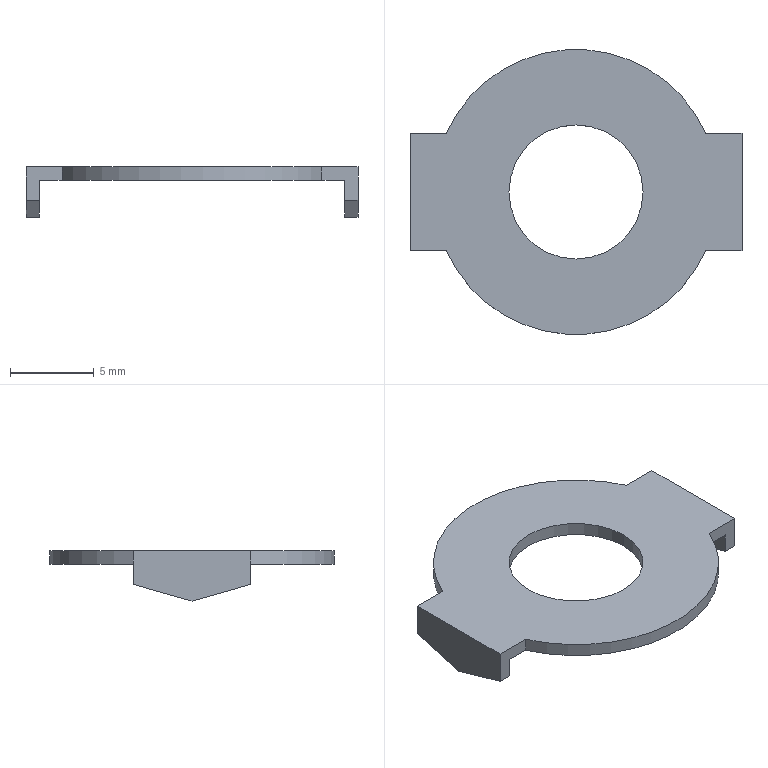Part | SolidWorks | features BaseBody 1 | 1 solid | 18 faces | box 19.8 x 17 x 3 mm | volume 178.855 mm3 | plane 14 | cylinder 4 | commonest cylinder face diameters 8 x2 17 x2
STEP:
#1=CARTESIAN_POINT('',(-4.,0.,-0.8));
#2=VERTEX_POINT('',#1);
#3=CARTESIAN_POINT('',(4.,0.,-0.8));
#4=VERTEX_POINT('',#3);
#5=CARTESIAN_POINT('',(0.,0.,-0.8));
#6=DIRECTION('',(0.,0.,1.));
#7=DIRECTION('',(1.,0.,0.));
#8=AXIS2_PLACEMENT_3D('',#5,#6,#7);
#9=CIRCLE('',#8,4.);
#10=EDGE_CURVE('',#2,#4,#9,.T.);
#11=ORIENTED_EDGE('',*,*,#10,.F.);
#12=CARTESIAN_POINT('',(-4.,0.,0.));
#13=VERTEX_POINT('',#12);
#14=CARTESIAN_POINT('',(-4.,0.,-3.));
#15=DIRECTION('',(0.,0.,1.));
#16=VECTOR('',#15,1000.);
#17=LINE('',#14,#16);
#18=EDGE_CURVE('',#2,#13,#17,.T.);
#19=ORIENTED_EDGE('',*,*,#18,.T.);
#20=CARTESIAN_POINT('',(4.,0.,0.));
#21=VERTEX_POINT('',#20);
#22=CARTESIAN_POINT('',(0.,0.,0.));
#23=DIRECTION('',(0.,0.,1.));
#24=DIRECTION('',(1.,0.,0.));
#25=AXIS2_PLACEMENT_3D('',#22,#23,#24);
#26=CIRCLE('',#25,4.);
#27=EDGE_CURVE('',#13,#21,#26,.T.);
#28=ORIENTED_EDGE('',*,*,#27,.T.);
#29=CARTESIAN_POINT('',(4.,0.,-3.));
#30=DIRECTION('',(0.,0.,1.));
#31=VECTOR('',#30,1000.);
#32=LINE('',#29,#31);
#33=EDGE_CURVE('',#4,#21,#32,.T.);
#34=ORIENTED_EDGE('',*,*,#33,.F.);
#35=EDGE_LOOP('',(#11,#19,#28,#34));
#36=FACE_OUTER_BOUND('',#35,.T.);
#37=CARTESIAN_POINT('',(0.,0.,-3.));
#38=DIRECTION('',(0.,0.,1.));
#39=DIRECTION('',(1.,0.,0.));
#40=AXIS2_PLACEMENT_3D('',#37,#38,#39);
#41=CYLINDRICAL_SURFACE('',#40,4.);
#42=ADVANCED_FACE('',(#36),#41,.F.);
#43=CARTESIAN_POINT('',(0.,0.,-0.8));
#44=DIRECTION('',(0.,0.,1.));
#45=DIRECTION('',(1.,0.,0.));
#46=AXIS2_PLACEMENT_3D('',#43,#44,#45);
#47=CIRCLE('',#46,4.);
#48=EDGE_CURVE('',#4,#2,#47,.T.);
#49=ORIENTED_EDGE('',*,*,#48,.T.);
#50=ORIENTED_EDGE('',*,*,#10,.T.);
#51=EDGE_LOOP('',(#49,#50));
#52=FACE_BOUND('',#51,.T.);
#53=CARTESIAN_POINT('',(-9.1,3.5,-0.8));
#54=VERTEX_POINT('',#53);
#55=CARTESIAN_POINT('',(-9.1,-3.5,-0.8));
#56=VERTEX_POINT('',#55);
#57=CARTESIAN_POINT('',(-9.1,0.,-0.8));
#58=DIRECTION('',(0.,-1.,0.));
#59=VECTOR('',#58,1000.);
#60=LINE('',#57,#59);
#61=EDGE_CURVE('',#54,#56,#60,.T.);
#62=ORIENTED_EDGE('',*,*,#61,.F.);
#63=CARTESIAN_POINT('',(-7.746,3.5,-0.8));
#64=VERTEX_POINT('',#63);
#65=CARTESIAN_POINT('',(-9.9,3.5,-0.8));
#66=DIRECTION('',(-1.,0.,0.));
#67=VECTOR('',#66,1000.);
#68=LINE('',#65,#67);
#69=EDGE_CURVE('',#64,#54,#68,.T.);
#70=ORIENTED_EDGE('',*,*,#69,.F.);
#71=CARTESIAN_POINT('',(7.746,3.5,-0.8));
#72=VERTEX_POINT('',#71);
#73=CARTESIAN_POINT('',(0.,0.,-0.8));
#74=DIRECTION('',(0.,0.,1.));
#75=DIRECTION('',(1.,0.,0.));
#76=AXIS2_PLACEMENT_3D('',#73,#74,#75);
#77=CIRCLE('',#76,8.5);
#78=EDGE_CURVE('',#72,#64,#77,.T.);
#79=ORIENTED_EDGE('',*,*,#78,.F.);
#80=CARTESIAN_POINT('',(9.1,3.5,-0.8));
#81=VERTEX_POINT('',#80);
#82=CARTESIAN_POINT('',(7.746,3.5,-0.8));
#83=DIRECTION('',(-1.,0.,0.));
#84=VECTOR('',#83,1000.);
#85=LINE('',#82,#84);
#86=EDGE_CURVE('',#81,#72,#85,.T.);
#87=ORIENTED_EDGE('',*,*,#86,.F.);
#88=CARTESIAN_POINT('',(9.1,-3.5,-0.8));
#89=VERTEX_POINT('',#88);
#90=CARTESIAN_POINT('',(9.1,0.,-0.8));
#91=DIRECTION('',(0.,1.,0.));
#92=VECTOR('',#91,1000.);
#93=LINE('',#90,#92);
#94=EDGE_CURVE('',#89,#81,#93,.T.);
#95=ORIENTED_EDGE('',*,*,#94,.F.);
#96=CARTESIAN_POINT('',(7.746,-3.5,-0.8));
#97=VERTEX_POINT('',#96);
#98=CARTESIAN_POINT('',(7.746,-3.5,-0.8));
#99=DIRECTION('',(1.,0.,0.));
#100=VECTOR('',#99,1000.);
#101=LINE('',#98,#100);
#102=EDGE_CURVE('',#97,#89,#101,.T.);
#103=ORIENTED_EDGE('',*,*,#102,.F.);
#104=CARTESIAN_POINT('',(-7.746,-3.5,-0.8));
#105=VERTEX_POINT('',#104);
#106=CARTESIAN_POINT('',(0.,0.,-0.8));
#107=DIRECTION('',(0.,0.,1.));
#108=DIRECTION('',(1.,0.,0.));
#109=AXIS2_PLACEMENT_3D('',#106,#107,#108);
#110=CIRCLE('',#109,8.5);
#111=EDGE_CURVE('',#105,#97,#110,.T.);
#112=ORIENTED_EDGE('',*,*,#111,.F.);
#113=CARTESIAN_POINT('',(-9.9,-3.5,-0.8));
#114=DIRECTION('',(1.,0.,0.));
#115=VECTOR('',#114,1000.);
#116=LINE('',#113,#115);
#117=EDGE_CURVE('',#56,#105,#116,.T.);
#118=ORIENTED_EDGE('',*,*,#117,.F.);
#119=EDGE_LOOP('',(#62,#70,#79,#87,#95,#103,#112,#118));
#120=FACE_OUTER_BOUND('',#119,.T.);
#121=CARTESIAN_POINT('',(0.,0.,-0.8));
#122=DIRECTION('',(0.,0.,1.));
#123=DIRECTION('',(1.,0.,0.));
#124=AXIS2_PLACEMENT_3D('',#121,#122,#123);
#125=PLANE('',#124);
#126=ADVANCED_FACE('',(#52,#120),#125,.F.);
#127=CARTESIAN_POINT('',(-7.746,-3.5,0.));
#128=VERTEX_POINT('',#127);
#129=CARTESIAN_POINT('',(7.746,-3.5,0.));
#130=VERTEX_POINT('',#129);
#131=CARTESIAN_POINT('',(0.,0.,0.));
#132=DIRECTION('',(0.,0.,1.));
#133=DIRECTION('',(1.,0.,0.));
#134=AXIS2_PLACEMENT_3D('',#131,#132,#133);
#135=CIRCLE('',#134,8.5);
#136=EDGE_CURVE('',#128,#130,#135,.T.);
#137=ORIENTED_EDGE('',*,*,#136,.F.);
#138=CARTESIAN_POINT('',(-7.746,-3.5,-0.8));
#139=DIRECTION('',(0.,0.,1.));
#140=VECTOR('',#139,1000.);
#141=LINE('',#138,#140);
#142=EDGE_CURVE('',#105,#128,#141,.T.);
#143=ORIENTED_EDGE('',*,*,#142,.F.);
#144=ORIENTED_EDGE('',*,*,#111,.T.);
#145=CARTESIAN_POINT('',(7.746,-3.5,-0.8));
#146=DIRECTION('',(0.,0.,1.));
#147=VECTOR('',#146,1000.);
#148=LINE('',#145,#147);
#149=EDGE_CURVE('',#97,#130,#148,.T.);
#150=ORIENTED_EDGE('',*,*,#149,.T.);
#151=EDGE_LOOP('',(#137,#143,#144,#150));
#152=FACE_OUTER_BOUND('',#151,.T.);
#153=CARTESIAN_POINT('',(0.,0.,-0.8));
#154=DIRECTION('',(0.,0.,1.));
#155=DIRECTION('',(1.,0.,0.));
#156=AXIS2_PLACEMENT_3D('',#153,#154,#155);
#157=CYLINDRICAL_SURFACE('',#156,8.5);
#158=ADVANCED_FACE('',(#152),#157,.T.);
#159=CARTESIAN_POINT('',(-9.9,-3.5,-2.));
#160=VERTEX_POINT('',#159);
#161=CARTESIAN_POINT('',(-9.9,-3.5,0.));
#162=VERTEX_POINT('',#161);
#163=CARTESIAN_POINT('',(-9.9,-3.5,-0.8));
#164=DIRECTION('',(0.,0.,1.));
#165=VECTOR('',#164,1000.);
#166=LINE('',#163,#165);
#167=EDGE_CURVE('',#160,#162,#166,.T.);
#168=ORIENTED_EDGE('',*,*,#167,.F.);
#169=CARTESIAN_POINT('',(-9.1,-3.5,-2.));
#170=VERTEX_POINT('',#169);
#171=CARTESIAN_POINT('',(-9.1,-3.5,-2.));
#172=DIRECTION('',(-1.,0.,0.));
#173=VECTOR('',#172,1000.);
#174=LINE('',#171,#173);
#175=EDGE_CURVE('',#170,#160,#174,.T.);
#176=ORIENTED_EDGE('',*,*,#175,.F.);
#177=CARTESIAN_POINT('',(-9.1,-3.5,0.));
#178=DIRECTION('',(0.,0.,-1.));
#179=VECTOR('',#178,1000.);
#180=LINE('',#177,#179);
#181=EDGE_CURVE('',#56,#170,#180,.T.);
#182=ORIENTED_EDGE('',*,*,#181,.F.);
#183=ORIENTED_EDGE('',*,*,#117,.T.);
#184=ORIENTED_EDGE('',*,*,#142,.T.);
#185=CARTESIAN_POINT('',(-9.9,-3.5,0.));
#186=DIRECTION('',(1.,0.,0.));
#187=VECTOR('',#186,1000.);
#188=LINE('',#185,#187);
#189=EDGE_CURVE('',#162,#128,#188,.T.);
#190=ORIENTED_EDGE('',*,*,#189,.F.);
#191=EDGE_LOOP('',(#168,#176,#182,#183,#184,#190));
#192=FACE_OUTER_BOUND('',#191,.T.);
#193=CARTESIAN_POINT('',(-9.9,-3.5,-0.8));
#194=DIRECTION('',(0.,-1.,0.));
#195=DIRECTION('',(1.,0.,0.));
#196=AXIS2_PLACEMENT_3D('',#193,#194,#195);
#197=PLANE('',#196);
#198=ADVANCED_FACE('',(#192),#197,.T.);
#199=CARTESIAN_POINT('',(-9.9,3.5,0.));
#200=VERTEX_POINT('',#199);
#201=CARTESIAN_POINT('',(-9.9,3.5,0.));
#202=DIRECTION('',(0.,-1.,0.));
#203=VECTOR('',#202,1000.);
#204=LINE('',#201,#203);
#205=EDGE_CURVE('',#200,#162,#204,.T.);
#206=ORIENTED_EDGE('',*,*,#205,.F.);
#207=CARTESIAN_POINT('',(-9.9,3.5,-2.));
#208=VERTEX_POINT('',#207);
#209=CARTESIAN_POINT('',(-9.9,3.5,-0.8));
#210=DIRECTION('',(0.,0.,1.));
#211=VECTOR('',#210,1000.);
#212=LINE('',#209,#211);
#213=EDGE_CURVE('',#208,#200,#212,.T.);
#214=ORIENTED_EDGE('',*,*,#213,.F.);
#215=CARTESIAN_POINT('',(-9.9,0.,-3.));
#216=VERTEX_POINT('',#215);
#217=CARTESIAN_POINT('',(-9.9,3.5,-2.));
#218=DIRECTION('',(0.,0.9615,0.2747));
#219=VECTOR('',#218,1000.);
#220=LINE('',#217,#219);
#221=EDGE_CURVE('',#216,#208,#220,.T.);
#222=ORIENTED_EDGE('',*,*,#221,.F.);
#223=CARTESIAN_POINT('',(-9.9,-3.5,-2.));
#224=DIRECTION('',(0.,0.9615,-0.2747));
#225=VECTOR('',#224,1000.);
#226=LINE('',#223,#225);
#227=EDGE_CURVE('',#160,#216,#226,.T.);
#228=ORIENTED_EDGE('',*,*,#227,.F.);
#229=ORIENTED_EDGE('',*,*,#167,.T.);
#230=EDGE_LOOP('',(#206,#214,#222,#228,#229));
#231=FACE_OUTER_BOUND('',#230,.T.);
#232=CARTESIAN_POINT('',(-9.9,3.5,-0.8));
#233=DIRECTION('',(-1.,0.,0.));
#234=DIRECTION('',(0.,0.,1.));
#235=AXIS2_PLACEMENT_3D('',#232,#233,#234);
#236=PLANE('',#235);
#237=ADVANCED_FACE('',(#231),#236,.T.);
#238=ORIENTED_EDGE('',*,*,#213,.T.);
#239=CARTESIAN_POINT('',(-7.746,3.5,0.));
#240=VERTEX_POINT('',#239);
#241=CARTESIAN_POINT('',(-9.9,3.5,0.));
#242=DIRECTION('',(-1.,0.,0.));
#243=VECTOR('',#242,1000.);
#244=LINE('',#241,#243);
#245=EDGE_CURVE('',#240,#200,#244,.T.);
#246=ORIENTED_EDGE('',*,*,#245,.F.);
#247=CARTESIAN_POINT('',(-7.746,3.5,-0.8));
#248=DIRECTION('',(0.,0.,1.));
#249=VECTOR('',#248,1000.);
#250=LINE('',#247,#249);
#251=EDGE_CURVE('',#64,#240,#250,.T.);
#252=ORIENTED_EDGE('',*,*,#251,.F.);
#253=ORIENTED_EDGE('',*,*,#69,.T.);
#254=CARTESIAN_POINT('',(-9.1,3.5,-2.));
#255=VERTEX_POINT('',#254);
#256=CARTESIAN_POINT('',(-9.1,3.5,0.));
#257=DIRECTION('',(0.,0.,1.));
#258=VECTOR('',#257,1000.);
#259=LINE('',#256,#258);
#260=EDGE_CURVE('',#255,#54,#259,.T.);
#261=ORIENTED_EDGE('',*,*,#260,.F.);
#262=CARTESIAN_POINT('',(-9.1,3.5,-2.));
#263=DIRECTION('',(-1.,0.,0.));
#264=VECTOR('',#263,1000.);
#265=LINE('',#262,#264);
#266=EDGE_CURVE('',#255,#208,#265,.T.);
#267=ORIENTED_EDGE('',*,*,#266,.T.);
#268=EDGE_LOOP('',(#238,#246,#252,#253,#261,#267));
#269=FACE_OUTER_BOUND('',#268,.T.);
#270=CARTESIAN_POINT('',(-9.9,3.5,-0.8));
#271=DIRECTION('',(0.,1.,0.));
#272=DIRECTION('',(-1.,0.,0.));
#273=AXIS2_PLACEMENT_3D('',#270,#271,#272);
#274=PLANE('',#273);
#275=ADVANCED_FACE('',(#269),#274,.T.);
#276=CARTESIAN_POINT('',(7.746,3.5,0.));
#277=VERTEX_POINT('',#276);
#278=CARTESIAN_POINT('',(0.,0.,0.));
#279=DIRECTION('',(0.,0.,1.));
#280=DIRECTION('',(1.,0.,0.));
#281=AXIS2_PLACEMENT_3D('',#278,#279,#280);
#282=CIRCLE('',#281,8.5);
#283=EDGE_CURVE('',#277,#240,#282,.T.);
#284=ORIENTED_EDGE('',*,*,#283,.F.);
#285=CARTESIAN_POINT('',(7.746,3.5,-0.8));
#286=DIRECTION('',(0.,0.,1.));
#287=VECTOR('',#286,1000.);
#288=LINE('',#285,#287);
#289=EDGE_CURVE('',#72,#277,#288,.T.);
#290=ORIENTED_EDGE('',*,*,#289,.F.);
#291=ORIENTED_EDGE('',*,*,#78,.T.);
#292=ORIENTED_EDGE('',*,*,#251,.T.);
#293=EDGE_LOOP('',(#284,#290,#291,#292));
#294=FACE_OUTER_BOUND('',#293,.T.);
#295=CARTESIAN_POINT('',(0.,0.,-0.8));
#296=DIRECTION('',(0.,0.,1.));
#297=DIRECTION('',(1.,0.,0.));
#298=AXIS2_PLACEMENT_3D('',#295,#296,#297);
#299=CYLINDRICAL_SURFACE('',#298,8.5);
#300=ADVANCED_FACE('',(#294),#299,.T.);
#301=CARTESIAN_POINT('',(9.1,3.5,-2.));
#302=VERTEX_POINT('',#301);
#303=CARTESIAN_POINT('',(9.1,3.5,0.));
#304=DIRECTION('',(0.,0.,1.));
#305=VECTOR('',#304,1000.);
#306=LINE('',#303,#305);
#307=EDGE_CURVE('',#302,#81,#306,.T.);
#308=ORIENTED_EDGE('',*,*,#307,.T.);
#309=ORIENTED_EDGE('',*,*,#86,.T.);
#310=ORIENTED_EDGE('',*,*,#289,.T.);
#311=CARTESIAN_POINT('',(9.9,3.5,0.));
#312=VERTEX_POINT('',#311);
#313=CARTESIAN_POINT('',(7.746,3.5,0.));
#314=DIRECTION('',(-1.,0.,0.));
#315=VECTOR('',#314,1000.);
#316=LINE('',#313,#315);
#317=EDGE_CURVE('',#312,#277,#316,.T.);
#318=ORIENTED_EDGE('',*,*,#317,.F.);
#319=CARTESIAN_POINT('',(9.9,3.5,-2.));
#320=VERTEX_POINT('',#319);
#321=CARTESIAN_POINT('',(9.9,3.5,-0.8));
#322=DIRECTION('',(0.,0.,1.));
#323=VECTOR('',#322,1000.);
#324=LINE('',#321,#323);
#325=EDGE_CURVE('',#320,#312,#324,.T.);
#326=ORIENTED_EDGE('',*,*,#325,.F.);
#327=CARTESIAN_POINT('',(9.1,3.5,-2.));
#328=DIRECTION('',(1.,0.,0.));
#329=VECTOR('',#328,1000.);
#330=LINE('',#327,#329);
#331=EDGE_CURVE('',#302,#320,#330,.T.);
#332=ORIENTED_EDGE('',*,*,#331,.F.);
#333=EDGE_LOOP('',(#308,#309,#310,#318,#326,#332));
#334=FACE_OUTER_BOUND('',#333,.T.);
#335=CARTESIAN_POINT('',(7.746,3.5,-0.8));
#336=DIRECTION('',(0.,1.,0.));
#337=DIRECTION('',(-1.,0.,0.));
#338=AXIS2_PLACEMENT_3D('',#335,#336,#337);
#339=PLANE('',#338);
#340=ADVANCED_FACE('',(#334),#339,.T.);
#341=CARTESIAN_POINT('',(9.9,-3.5,0.));
#342=VERTEX_POINT('',#341);
#343=CARTESIAN_POINT('',(9.9,3.5,0.));
#344=DIRECTION('',(0.,1.,0.));
#345=VECTOR('',#344,1000.);
#346=LINE('',#343,#345);
#347=EDGE_CURVE('',#342,#312,#346,.T.);
#348=ORIENTED_EDGE('',*,*,#347,.F.);
#349=CARTESIAN_POINT('',(9.9,-3.5,-2.));
#350=VERTEX_POINT('',#349);
#351=CARTESIAN_POINT('',(9.9,-3.5,-0.8));
#352=DIRECTION('',(0.,0.,1.));
#353=VECTOR('',#352,1000.);
#354=LINE('',#351,#353);
#355=EDGE_CURVE('',#350,#342,#354,.T.);
#356=ORIENTED_EDGE('',*,*,#355,.F.);
#357=CARTESIAN_POINT('',(9.9,0.,-3.));
#358=VERTEX_POINT('',#357);
#359=CARTESIAN_POINT('',(9.9,-3.5,-2.));
#360=DIRECTION('',(0.,0.9615,-0.2747));
#361=VECTOR('',#360,1000.);
#362=LINE('',#359,#361);
#363=EDGE_CURVE('',#350,#358,#362,.T.);
#364=ORIENTED_EDGE('',*,*,#363,.T.);
#365=CARTESIAN_POINT('',(9.9,3.5,-2.));
#366=DIRECTION('',(0.,0.9615,0.2747));
#367=VECTOR('',#366,1000.);
#368=LINE('',#365,#367);
#369=EDGE_CURVE('',#358,#320,#368,.T.);
#370=ORIENTED_EDGE('',*,*,#369,.T.);
#371=ORIENTED_EDGE('',*,*,#325,.T.);
#372=EDGE_LOOP('',(#348,#356,#364,#370,#371));
#373=FACE_OUTER_BOUND('',#372,.T.);
#374=CARTESIAN_POINT('',(9.9,3.5,-0.8));
#375=DIRECTION('',(1.,0.,0.));
#376=DIRECTION('',(0.,0.,-1.));
#377=AXIS2_PLACEMENT_3D('',#374,#375,#376);
#378=PLANE('',#377);
#379=ADVANCED_FACE('',(#373),#378,.T.);
#380=ORIENTED_EDGE('',*,*,#355,.T.);
#381=CARTESIAN_POINT('',(7.746,-3.5,0.));
#382=DIRECTION('',(1.,0.,0.));
#383=VECTOR('',#382,1000.);
#384=LINE('',#381,#383);
#385=EDGE_CURVE('',#130,#342,#384,.T.);
#386=ORIENTED_EDGE('',*,*,#385,.F.);
#387=ORIENTED_EDGE('',*,*,#149,.F.);
#388=ORIENTED_EDGE('',*,*,#102,.T.);
#389=CARTESIAN_POINT('',(9.1,-3.5,-2.));
#390=VERTEX_POINT('',#389);
#391=CARTESIAN_POINT('',(9.1,-3.5,0.));
#392=DIRECTION('',(0.,0.,-1.));
#393=VECTOR('',#392,1000.);
#394=LINE('',#391,#393);
#395=EDGE_CURVE('',#89,#390,#394,.T.);
#396=ORIENTED_EDGE('',*,*,#395,.T.);
#397=CARTESIAN_POINT('',(9.1,-3.5,-2.));
#398=DIRECTION('',(1.,0.,0.));
#399=VECTOR('',#398,1000.);
#400=LINE('',#397,#399);
#401=EDGE_CURVE('',#390,#350,#400,.T.);
#402=ORIENTED_EDGE('',*,*,#401,.T.);
#403=EDGE_LOOP('',(#380,#386,#387,#388,#396,#402));
#404=FACE_OUTER_BOUND('',#403,.T.);
#405=CARTESIAN_POINT('',(7.746,-3.5,-0.8));
#406=DIRECTION('',(0.,-1.,0.));
#407=DIRECTION('',(1.,0.,0.));
#408=AXIS2_PLACEMENT_3D('',#405,#406,#407);
#409=PLANE('',#408);
#410=ADVANCED_FACE('',(#404),#409,.T.);
#411=CARTESIAN_POINT('',(0.,0.,0.));
#412=DIRECTION('',(0.,0.,1.));
#413=DIRECTION('',(1.,0.,0.));
#414=AXIS2_PLACEMENT_3D('',#411,#412,#413);
#415=CIRCLE('',#414,4.);
#416=EDGE_CURVE('',#21,#13,#415,.T.);
#417=ORIENTED_EDGE('',*,*,#416,.F.);
#418=ORIENTED_EDGE('',*,*,#27,.F.);
#419=EDGE_LOOP('',(#417,#418));
#420=FACE_BOUND('',#419,.T.);
#421=ORIENTED_EDGE('',*,*,#189,.T.);
#422=ORIENTED_EDGE('',*,*,#136,.T.);
#423=ORIENTED_EDGE('',*,*,#385,.T.);
#424=ORIENTED_EDGE('',*,*,#347,.T.);
#425=ORIENTED_EDGE('',*,*,#317,.T.);
#426=ORIENTED_EDGE('',*,*,#283,.T.);
#427=ORIENTED_EDGE('',*,*,#245,.T.);
#428=ORIENTED_EDGE('',*,*,#205,.T.);
#429=EDGE_LOOP('',(#421,#422,#423,#424,#425,#426,#427,#428));
#430=FACE_OUTER_BOUND('',#429,.T.);
#431=CARTESIAN_POINT('',(0.,0.,0.));
#432=DIRECTION('',(0.,0.,1.));
#433=DIRECTION('',(1.,0.,0.));
#434=AXIS2_PLACEMENT_3D('',#431,#432,#433);
#435=PLANE('',#434);
#436=ADVANCED_FACE('',(#420,#430),#435,.T.);
#437=ORIENTED_EDGE('',*,*,#395,.F.);
#438=ORIENTED_EDGE('',*,*,#94,.T.);
#439=ORIENTED_EDGE('',*,*,#307,.F.);
#440=CARTESIAN_POINT('',(9.1,0.,-3.));
#441=VERTEX_POINT('',#440);
#442=CARTESIAN_POINT('',(9.1,3.5,-2.));
#443=DIRECTION('',(0.,0.9615,0.2747));
#444=VECTOR('',#443,1000.);
#445=LINE('',#442,#444);
#446=EDGE_CURVE('',#441,#302,#445,.T.);
#447=ORIENTED_EDGE('',*,*,#446,.F.);
#448=CARTESIAN_POINT('',(9.1,-3.5,-2.));
#449=DIRECTION('',(0.,0.9615,-0.2747));
#450=VECTOR('',#449,1000.);
#451=LINE('',#448,#450);
#452=EDGE_CURVE('',#390,#441,#451,.T.);
#453=ORIENTED_EDGE('',*,*,#452,.F.);
#454=EDGE_LOOP('',(#437,#438,#439,#447,#453));
#455=FACE_OUTER_BOUND('',#454,.T.);
#456=CARTESIAN_POINT('',(9.1,-3.5,0.));
#457=DIRECTION('',(1.,0.,0.));
#458=DIRECTION('',(0.,0.,-1.));
#459=AXIS2_PLACEMENT_3D('',#456,#457,#458);
#460=PLANE('',#459);
#461=ADVANCED_FACE('',(#455),#460,.F.);
#462=ORIENTED_EDGE('',*,*,#369,.F.);
#463=CARTESIAN_POINT('',(9.1,0.,-3.));
#464=DIRECTION('',(1.,0.,0.));
#465=VECTOR('',#464,1000.);
#466=LINE('',#463,#465);
#467=EDGE_CURVE('',#441,#358,#466,.T.);
#468=ORIENTED_EDGE('',*,*,#467,.F.);
#469=ORIENTED_EDGE('',*,*,#446,.T.);
#470=ORIENTED_EDGE('',*,*,#331,.T.);
#471=EDGE_LOOP('',(#462,#468,#469,#470));
#472=FACE_OUTER_BOUND('',#471,.T.);
#473=CARTESIAN_POINT('',(9.1,3.5,-2.));
#474=DIRECTION('',(0.,0.2747,-0.9615));
#475=DIRECTION('',(0.,0.9615,0.2747));
#476=AXIS2_PLACEMENT_3D('',#473,#474,#475);
#477=PLANE('',#476);
#478=ADVANCED_FACE('',(#472),#477,.T.);
#479=ORIENTED_EDGE('',*,*,#363,.F.);
#480=ORIENTED_EDGE('',*,*,#401,.F.);
#481=ORIENTED_EDGE('',*,*,#452,.T.);
#482=ORIENTED_EDGE('',*,*,#467,.T.);
#483=EDGE_LOOP('',(#479,#480,#481,#482));
#484=FACE_OUTER_BOUND('',#483,.T.);
#485=CARTESIAN_POINT('',(9.1,-3.5,-2.));
#486=DIRECTION('',(0.,-0.2747,-0.9615));
#487=DIRECTION('',(0.,0.9615,-0.2747));
#488=AXIS2_PLACEMENT_3D('',#485,#486,#487);
#489=PLANE('',#488);
#490=ADVANCED_FACE('',(#484),#489,.T.);
#491=ORIENTED_EDGE('',*,*,#260,.T.);
#492=ORIENTED_EDGE('',*,*,#61,.T.);
#493=ORIENTED_EDGE('',*,*,#181,.T.);
#494=CARTESIAN_POINT('',(-9.1,0.,-3.));
#495=VERTEX_POINT('',#494);
#496=CARTESIAN_POINT('',(-9.1,-3.5,-2.));
#497=DIRECTION('',(0.,0.9615,-0.2747));
#498=VECTOR('',#497,1000.);
#499=LINE('',#496,#498);
#500=EDGE_CURVE('',#170,#495,#499,.T.);
#501=ORIENTED_EDGE('',*,*,#500,.T.);
#502=CARTESIAN_POINT('',(-9.1,3.5,-2.));
#503=DIRECTION('',(0.,0.9615,0.2747));
#504=VECTOR('',#503,1000.);
#505=LINE('',#502,#504);
#506=EDGE_CURVE('',#495,#255,#505,.T.);
#507=ORIENTED_EDGE('',*,*,#506,.T.);
#508=EDGE_LOOP('',(#491,#492,#493,#501,#507));
#509=FACE_OUTER_BOUND('',#508,.T.);
#510=CARTESIAN_POINT('',(-9.1,-3.5,0.));
#511=DIRECTION('',(-1.,0.,0.));
#512=DIRECTION('',(0.,0.,-1.));
#513=AXIS2_PLACEMENT_3D('',#510,#511,#512);
#514=PLANE('',#513);
#515=ADVANCED_FACE('',(#509),#514,.F.);
#516=ORIENTED_EDGE('',*,*,#227,.T.);
#517=CARTESIAN_POINT('',(-9.1,0.,-3.));
#518=DIRECTION('',(-1.,0.,0.));
#519=VECTOR('',#518,1000.);
#520=LINE('',#517,#519);
#521=EDGE_CURVE('',#495,#216,#520,.T.);
#522=ORIENTED_EDGE('',*,*,#521,.F.);
#523=ORIENTED_EDGE('',*,*,#500,.F.);
#524=ORIENTED_EDGE('',*,*,#175,.T.);
#525=EDGE_LOOP('',(#516,#522,#523,#524));
#526=FACE_OUTER_BOUND('',#525,.T.);
#527=CARTESIAN_POINT('',(-9.1,-3.5,-2.));
#528=DIRECTION('',(0.,0.2747,0.9615));
#529=DIRECTION('',(0.,-0.9615,0.2747));
#530=AXIS2_PLACEMENT_3D('',#527,#528,#529);
#531=PLANE('',#530);
#532=ADVANCED_FACE('',(#526),#531,.F.);
#533=ORIENTED_EDGE('',*,*,#221,.T.);
#534=ORIENTED_EDGE('',*,*,#266,.F.);
#535=ORIENTED_EDGE('',*,*,#506,.F.);
#536=ORIENTED_EDGE('',*,*,#521,.T.);
#537=EDGE_LOOP('',(#533,#534,#535,#536));
#538=FACE_OUTER_BOUND('',#537,.T.);
#539=CARTESIAN_POINT('',(-9.1,3.5,-2.));
#540=DIRECTION('',(0.,-0.2747,0.9615));
#541=DIRECTION('',(0.,-0.9615,-0.2747));
#542=AXIS2_PLACEMENT_3D('',#539,#540,#541);
#543=PLANE('',#542);
#544=ADVANCED_FACE('',(#538),#543,.F.);
#545=ORIENTED_EDGE('',*,*,#18,.F.);
#546=ORIENTED_EDGE('',*,*,#48,.F.);
#547=ORIENTED_EDGE('',*,*,#33,.T.);
#548=ORIENTED_EDGE('',*,*,#416,.T.);
#549=EDGE_LOOP('',(#545,#546,#547,#548));
#550=FACE_OUTER_BOUND('',#549,.T.);
#551=CARTESIAN_POINT('',(0.,0.,-3.));
#552=DIRECTION('',(0.,0.,1.));
#553=DIRECTION('',(1.,0.,0.));
#554=AXIS2_PLACEMENT_3D('',#551,#552,#553);
#555=CYLINDRICAL_SURFACE('',#554,4.);
#556=ADVANCED_FACE('',(#550),#555,.F.);
#557=CLOSED_SHELL('',(#42,#126,#158,#198,#237,#275,#300,#340,#379,#410,#436,#461,#478,#490,#515,#532,#544,#556));
#558=MANIFOLD_SOLID_BREP('',#557);
#559=CARTESIAN_POINT('',(0.,0.,0.));
#560=DIRECTION('',(0.,0.,1.));
#561=DIRECTION('',(1.,0.,0.));
#562=AXIS2_PLACEMENT_3D('',#559,#560,#561);
#563=(LENGTH_UNIT()NAMED_UNIT(*)SI_UNIT(.MILLI.,.METRE.));
#564=UNCERTAINTY_MEASURE_WITH_UNIT(LENGTH_MEASURE(0.00001),#563,'','');
#565=(NAMED_UNIT(*)PLANE_ANGLE_UNIT()SI_UNIT($,.RADIAN.));
#566=(NAMED_UNIT(*)SI_UNIT($,.STERADIAN.)SOLID_ANGLE_UNIT());
#567=(GEOMETRIC_REPRESENTATION_CONTEXT(3)GLOBAL_UNCERTAINTY_ASSIGNED_CONTEXT((#564))GLOBAL_UNIT_ASSIGNED_CONTEXT((#563,#565,#566))REPRESENTATION_CONTEXT('',''));
#568=ADVANCED_BREP_SHAPE_REPRESENTATION('',(#558,#562),#567);